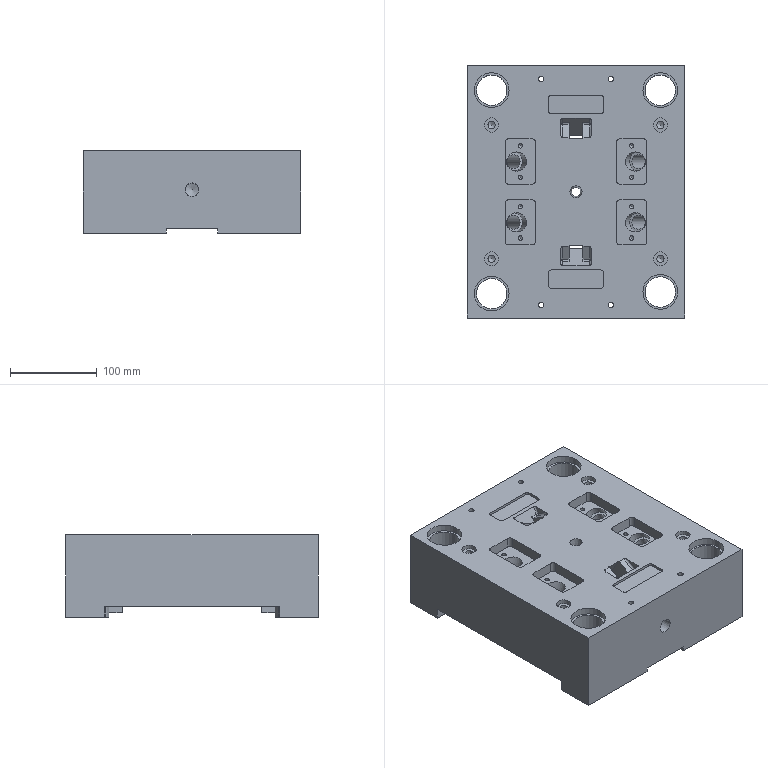Part | STEP file | AA_id278_x_t | 1 solid | 264 faces | box 250 x 290 x 95 mm | volume 4489597 mm3 | plane 117 | cylinder 112 | cone 27 | sphere 4 | torus 4 | commonest cylinder face diameters 8 x24 6 x16 4 x12 5 x12 16 x10 10 x8